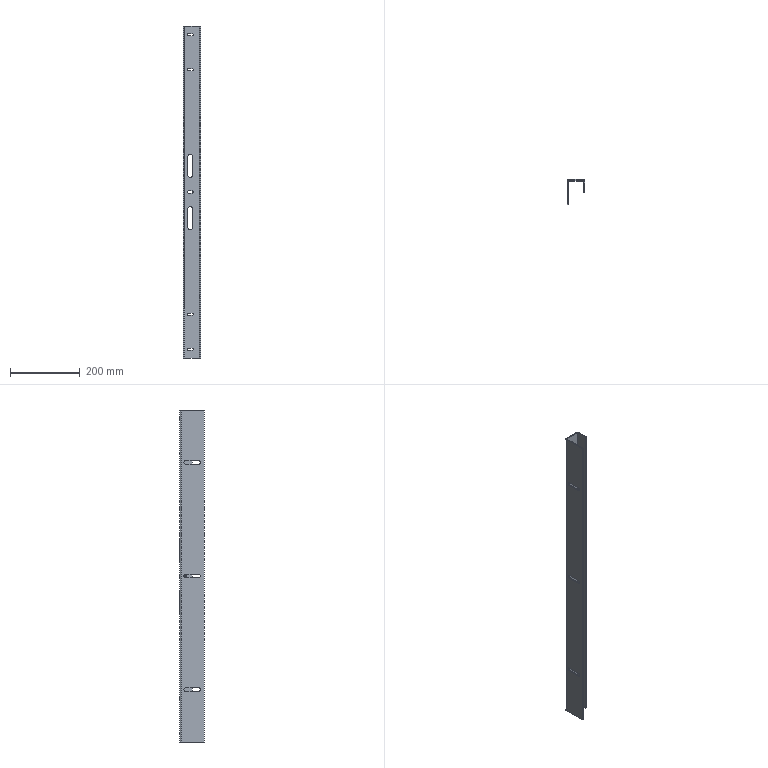Part | 1 solid | 73 faces | box 50 x 70 x 950 mm | volume 407445 mm3 | plane 38 | cylinder 35 | commonest cylinder face diameters 6 x15 7 x6 10 x6 14 x4 2 x2 8 x2